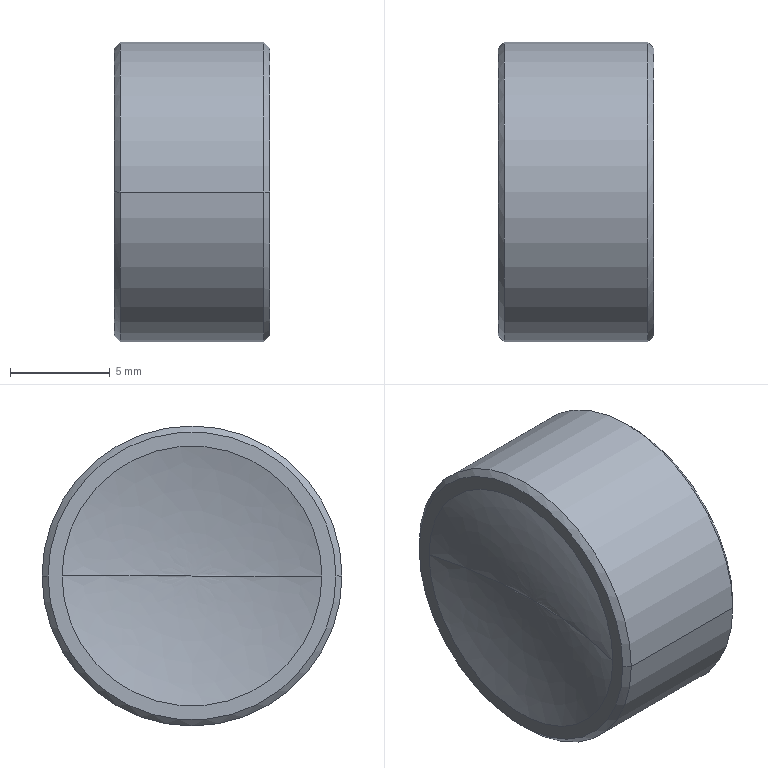Part | STEP file | biconcave lens 4.stp.STEP-235.STEP | 1 solid | 12 faces | box 7.786 x 15 x 15 mm | volume 1252 mm3 | cone 4 | spline 2 | sphere 2 | cylinder 2 | plane 2 | commonest cylinder face diameters 15 x2
STEP:
#1=CARTESIAN_POINT('',(413.933,-0.000000003,0.));
#2=VERTEX_POINT('',#1);
#3=CARTESIAN_POINT('',(413.04,-6.5,0.));
#4=VERTEX_POINT('',#3);
#5=CARTESIAN_POINT('',(413.933,-0.000000003,0.));
#6=CARTESIAN_POINT('',(413.933,-2.201,0.));
#7=CARTESIAN_POINT('',(413.633,-4.381,0.));
#8=CARTESIAN_POINT('',(413.04,-6.5,0.));
#9=(BOUNDED_CURVE()B_SPLINE_CURVE(3,(#5,#6,#7,#8),.UNSPECIFIED.,.F.,.T.)B_SPLINE_CURVE_WITH_KNOTS((4,4),(0.,6.283),.UNSPECIFIED.)CURVE()GEOMETRIC_REPRESENTATION_ITEM()RATIONAL_B_SPLINE_CURVE((1.,0.9938,0.9938,1.))REPRESENTATION_ITEM(''));
#10=EDGE_CURVE('',#2,#4,#9,.T.);
#11=ORIENTED_EDGE('',*,*,#10,.F.);
#12=CARTESIAN_POINT('',(413.04,6.5,0.));
#13=VERTEX_POINT('',#12);
#14=CARTESIAN_POINT('',(413.933,-0.000000003,0.));
#15=CARTESIAN_POINT('',(413.933,2.201,0.));
#16=CARTESIAN_POINT('',(413.633,4.381,0.));
#17=CARTESIAN_POINT('',(413.04,6.5,0.));
#18=(BOUNDED_CURVE()B_SPLINE_CURVE(3,(#14,#15,#16,#17),.UNSPECIFIED.,.F.,.F.)B_SPLINE_CURVE_WITH_KNOTS((4,4),(0.,6.283),.UNSPECIFIED.)CURVE()GEOMETRIC_REPRESENTATION_ITEM()RATIONAL_B_SPLINE_CURVE((1.,0.9938,0.9938,1.))REPRESENTATION_ITEM(''));
#19=EDGE_CURVE('',#2,#13,#18,.T.);
#20=ORIENTED_EDGE('',*,*,#19,.T.);
#21=CARTESIAN_POINT('',(413.04,0.,0.));
#22=DIRECTION('',(1.,0.,0.));
#23=DIRECTION('',(0.,-1.,0.));
#24=AXIS2_PLACEMENT_3D('',#21,#22,#23);
#25=CIRCLE('',#24,6.5);
#26=EDGE_CURVE('',#4,#13,#25,.T.);
#27=ORIENTED_EDGE('',*,*,#26,.F.);
#28=EDGE_LOOP('',(#11,#20,#27));
#29=FACE_OUTER_BOUND('',#28,.T.);
#30=CARTESIAN_POINT('',(413.933,0.,0.));
#31=CARTESIAN_POINT('',(413.933,0.,0.));
#32=CARTESIAN_POINT('',(413.933,0.,0.));
#33=CARTESIAN_POINT('',(413.933,0.,0.));
#34=CARTESIAN_POINT('',(413.933,-2.201,0.));
#35=CARTESIAN_POINT('',(413.933,-2.201,-4.401));
#36=CARTESIAN_POINT('',(413.933,2.201,-4.401));
#37=CARTESIAN_POINT('',(413.933,2.201,0.));
#38=CARTESIAN_POINT('',(413.633,-4.381,0.));
#39=CARTESIAN_POINT('',(413.633,-4.381,-8.762));
#40=CARTESIAN_POINT('',(413.633,4.381,-8.762));
#41=CARTESIAN_POINT('',(413.633,4.381,0.));
#42=CARTESIAN_POINT('',(413.04,-6.5,0.));
#43=CARTESIAN_POINT('',(413.04,-6.5,-13.));
#44=CARTESIAN_POINT('',(413.04,6.5,-13.));
#45=CARTESIAN_POINT('',(413.04,6.5,0.));
#46=(BOUNDED_SURFACE()B_SPLINE_SURFACE(3,3,((#30,#31,#32,#33),(#34,#35,#36,#37),(#38,#39,#40,#41),(#42,#43,#44,#45)),.UNSPECIFIED.,.F.,.F.,.T.)B_SPLINE_SURFACE_WITH_KNOTS((4,4),(4,4),(0.,6.283),(1.298,1.434),.UNSPECIFIED.)GEOMETRIC_REPRESENTATION_ITEM()RATIONAL_B_SPLINE_SURFACE(((1.,0.3333,0.3333,1.),(0.9938,0.3313,0.3313,0.9938),(0.9938,0.3313,0.3313,0.9938),(1.,0.3333,0.3333,1.)))REPRESENTATION_ITEM('')SURFACE());
#47=ADVANCED_FACE('',(#29),#46,.F.);
#48=CARTESIAN_POINT('',(420.826,6.5,0.));
#49=VERTEX_POINT('',#48);
#50=CARTESIAN_POINT('',(420.826,-6.5,0.));
#51=VERTEX_POINT('',#50);
#52=CARTESIAN_POINT('',(444.032,0.,0.));
#53=DIRECTION('',(0.,0.,1.));
#54=DIRECTION('',(0.,-1.,0.));
#55=AXIS2_PLACEMENT_3D('',#52,#53,#54);
#56=CIRCLE('',#55,24.099);
#57=EDGE_CURVE('',#49,#51,#56,.T.);
#58=ORIENTED_EDGE('',*,*,#57,.F.);
#59=CARTESIAN_POINT('',(420.826,0.,0.));
#60=DIRECTION('',(1.,0.,0.));
#61=DIRECTION('',(0.,-1.,0.));
#62=AXIS2_PLACEMENT_3D('',#59,#60,#61);
#63=CIRCLE('',#62,6.5);
#64=EDGE_CURVE('',#49,#51,#63,.T.);
#65=ORIENTED_EDGE('',*,*,#64,.T.);
#66=EDGE_LOOP('',(#58,#65));
#67=FACE_OUTER_BOUND('',#66,.T.);
#68=CARTESIAN_POINT('',(444.032,0.,0.));
#69=DIRECTION('',(0.,0.,1.));
#70=DIRECTION('',(0.,-1.,0.));
#71=AXIS2_PLACEMENT_3D('',#68,#69,#70);
#72=SPHERICAL_SURFACE('',#71,24.099);
#73=ADVANCED_FACE('',(#67),#72,.F.);
#74=CARTESIAN_POINT('',(420.826,7.2,0.));
#75=VERTEX_POINT('',#74);
#76=CARTESIAN_POINT('',(420.826,-7.2,0.));
#77=VERTEX_POINT('',#76);
#78=CARTESIAN_POINT('',(420.826,0.,0.));
#79=DIRECTION('',(1.,0.,0.));
#80=DIRECTION('',(0.,1.,0.));
#81=AXIS2_PLACEMENT_3D('',#78,#79,#80);
#82=CIRCLE('',#81,7.2);
#83=EDGE_CURVE('',#75,#77,#82,.T.);
#84=ORIENTED_EDGE('',*,*,#83,.F.);
#85=CARTESIAN_POINT('',(420.526,7.5,0.));
#86=VERTEX_POINT('',#85);
#87=CARTESIAN_POINT('',(420.826,7.2,0.));
#88=DIRECTION('',(-0.7071,0.7071,0.));
#89=VECTOR('',#88,1000.);
#90=LINE('',#87,#89);
#91=EDGE_CURVE('',#75,#86,#90,.T.);
#92=ORIENTED_EDGE('',*,*,#91,.T.);
#93=CARTESIAN_POINT('',(420.526,-7.5,0.));
#94=VERTEX_POINT('',#93);
#95=CARTESIAN_POINT('',(420.526,0.,0.));
#96=DIRECTION('',(-1.,0.,0.));
#97=DIRECTION('',(0.,1.,0.));
#98=AXIS2_PLACEMENT_3D('',#95,#96,#97);
#99=CIRCLE('',#98,7.5);
#100=EDGE_CURVE('',#94,#86,#99,.T.);
#101=ORIENTED_EDGE('',*,*,#100,.F.);
#102=CARTESIAN_POINT('',(420.826,-7.2,0.));
#103=DIRECTION('',(-0.7071,-0.7071,0.));
#104=VECTOR('',#103,1000.);
#105=LINE('',#102,#104);
#106=EDGE_CURVE('',#77,#94,#105,.T.);
#107=ORIENTED_EDGE('',*,*,#106,.F.);
#108=EDGE_LOOP('',(#84,#92,#101,#107));
#109=FACE_OUTER_BOUND('',#108,.T.);
#110=CARTESIAN_POINT('',(420.826,0.,0.));
#111=DIRECTION('',(-1.,0.,0.));
#112=DIRECTION('',(0.,-1.,0.));
#113=AXIS2_PLACEMENT_3D('',#110,#111,#112);
#114=CONICAL_SURFACE('',#113,7.2,0.7854);
#115=ADVANCED_FACE('',(#109),#114,.T.);
#116=CARTESIAN_POINT('',(413.04,-7.2,0.));
#117=VERTEX_POINT('',#116);
#118=CARTESIAN_POINT('',(413.04,7.2,0.));
#119=VERTEX_POINT('',#118);
#120=CARTESIAN_POINT('',(413.04,0.,0.));
#121=DIRECTION('',(-1.,0.,0.));
#122=DIRECTION('',(0.,-1.,0.));
#123=AXIS2_PLACEMENT_3D('',#120,#121,#122);
#124=CIRCLE('',#123,7.2);
#125=EDGE_CURVE('',#117,#119,#124,.T.);
#126=ORIENTED_EDGE('',*,*,#125,.F.);
#127=CARTESIAN_POINT('',(413.34,-7.5,0.));
#128=VERTEX_POINT('',#127);
#129=CARTESIAN_POINT('',(413.34,-7.5,0.));
#130=DIRECTION('',(0.7071,-0.7071,0.));
#131=VECTOR('',#130,1000.);
#132=LINE('',#129,#131);
#133=EDGE_CURVE('',#117,#128,#132,.T.);
#134=ORIENTED_EDGE('',*,*,#133,.T.);
#135=CARTESIAN_POINT('',(413.34,7.5,0.));
#136=VERTEX_POINT('',#135);
#137=CARTESIAN_POINT('',(413.34,0.,0.));
#138=DIRECTION('',(1.,0.,0.));
#139=DIRECTION('',(0.,-1.,0.));
#140=AXIS2_PLACEMENT_3D('',#137,#138,#139);
#141=CIRCLE('',#140,7.5);
#142=EDGE_CURVE('',#136,#128,#141,.T.);
#143=ORIENTED_EDGE('',*,*,#142,.F.);
#144=CARTESIAN_POINT('',(413.34,7.5,0.));
#145=DIRECTION('',(0.7071,0.7071,0.));
#146=VECTOR('',#145,1000.);
#147=LINE('',#144,#146);
#148=EDGE_CURVE('',#119,#136,#147,.T.);
#149=ORIENTED_EDGE('',*,*,#148,.F.);
#150=EDGE_LOOP('',(#126,#134,#143,#149));
#151=FACE_OUTER_BOUND('',#150,.T.);
#152=CARTESIAN_POINT('',(413.34,0.,0.));
#153=DIRECTION('',(1.,0.,0.));
#154=DIRECTION('',(0.,1.,0.));
#155=AXIS2_PLACEMENT_3D('',#152,#153,#154);
#156=CONICAL_SURFACE('',#155,7.5,0.7854);
#157=ADVANCED_FACE('',(#151),#156,.T.);
#158=CARTESIAN_POINT('',(413.34,0.,0.));
#159=DIRECTION('',(1.,0.,0.));
#160=DIRECTION('',(0.,-1.,0.));
#161=AXIS2_PLACEMENT_3D('',#158,#159,#160);
#162=CIRCLE('',#161,7.5);
#163=EDGE_CURVE('',#128,#136,#162,.T.);
#164=ORIENTED_EDGE('',*,*,#163,.T.);
#165=CARTESIAN_POINT('',(0.,7.5,0.));
#166=DIRECTION('',(1.,0.,0.));
#167=VECTOR('',#166,1000.);
#168=LINE('',#165,#167);
#169=EDGE_CURVE('',#136,#86,#168,.T.);
#170=ORIENTED_EDGE('',*,*,#169,.T.);
#171=CARTESIAN_POINT('',(420.526,0.,0.));
#172=DIRECTION('',(-1.,0.,0.));
#173=DIRECTION('',(0.,1.,0.));
#174=AXIS2_PLACEMENT_3D('',#171,#172,#173);
#175=CIRCLE('',#174,7.5);
#176=EDGE_CURVE('',#86,#94,#175,.T.);
#177=ORIENTED_EDGE('',*,*,#176,.T.);
#178=CARTESIAN_POINT('',(0.,-7.5,0.));
#179=DIRECTION('',(1.,0.,0.));
#180=VECTOR('',#179,1000.);
#181=LINE('',#178,#180);
#182=EDGE_CURVE('',#128,#94,#181,.T.);
#183=ORIENTED_EDGE('',*,*,#182,.F.);
#184=EDGE_LOOP('',(#164,#170,#177,#183));
#185=FACE_OUTER_BOUND('',#184,.T.);
#186=CARTESIAN_POINT('',(0.,0.,0.));
#187=DIRECTION('',(1.,0.,0.));
#188=DIRECTION('',(0.,-1.,0.));
#189=AXIS2_PLACEMENT_3D('',#186,#187,#188);
#190=CYLINDRICAL_SURFACE('',#189,7.5);
#191=ADVANCED_FACE('',(#185),#190,.T.);
#192=ORIENTED_EDGE('',*,*,#26,.T.);
#193=CARTESIAN_POINT('',(413.04,0.,0.));
#194=DIRECTION('',(1.,0.,0.));
#195=DIRECTION('',(0.,-1.,0.));
#196=AXIS2_PLACEMENT_3D('',#193,#194,#195);
#197=CIRCLE('',#196,6.5);
#198=EDGE_CURVE('',#13,#4,#197,.T.);
#199=ORIENTED_EDGE('',*,*,#198,.T.);
#200=EDGE_LOOP('',(#192,#199));
#201=FACE_BOUND('',#200,.T.);
#202=CARTESIAN_POINT('',(413.04,0.,0.));
#203=DIRECTION('',(-1.,0.,0.));
#204=DIRECTION('',(0.,-1.,0.));
#205=AXIS2_PLACEMENT_3D('',#202,#203,#204);
#206=CIRCLE('',#205,7.2);
#207=EDGE_CURVE('',#119,#117,#206,.T.);
#208=ORIENTED_EDGE('',*,*,#207,.T.);
#209=ORIENTED_EDGE('',*,*,#125,.T.);
#210=EDGE_LOOP('',(#208,#209));
#211=FACE_OUTER_BOUND('',#210,.T.);
#212=CARTESIAN_POINT('',(413.04,7.5,0.));
#213=DIRECTION('',(-1.,0.,0.));
#214=DIRECTION('',(0.,1.,0.));
#215=AXIS2_PLACEMENT_3D('',#212,#213,#214);
#216=PLANE('',#215);
#217=ADVANCED_FACE('',(#201,#211),#216,.T.);
#218=ORIENTED_EDGE('',*,*,#169,.F.);
#219=ORIENTED_EDGE('',*,*,#142,.T.);
#220=ORIENTED_EDGE('',*,*,#182,.T.);
#221=ORIENTED_EDGE('',*,*,#100,.T.);
#222=EDGE_LOOP('',(#218,#219,#220,#221));
#223=FACE_OUTER_BOUND('',#222,.T.);
#224=CARTESIAN_POINT('',(0.,0.,0.));
#225=DIRECTION('',(1.,0.,0.));
#226=DIRECTION('',(0.,-1.,0.));
#227=AXIS2_PLACEMENT_3D('',#224,#225,#226);
#228=CYLINDRICAL_SURFACE('',#227,7.5);
#229=ADVANCED_FACE('',(#223),#228,.T.);
#230=ORIENTED_EDGE('',*,*,#19,.F.);
#231=ORIENTED_EDGE('',*,*,#10,.T.);
#232=ORIENTED_EDGE('',*,*,#198,.F.);
#233=EDGE_LOOP('',(#230,#231,#232));
#234=FACE_OUTER_BOUND('',#233,.T.);
#235=CARTESIAN_POINT('',(413.933,0.,0.));
#236=CARTESIAN_POINT('',(413.933,0.,0.));
#237=CARTESIAN_POINT('',(413.933,0.,0.));
#238=CARTESIAN_POINT('',(413.933,0.,0.));
#239=CARTESIAN_POINT('',(413.933,2.201,0.));
#240=CARTESIAN_POINT('',(413.933,2.201,4.401));
#241=CARTESIAN_POINT('',(413.933,-2.201,4.401));
#242=CARTESIAN_POINT('',(413.933,-2.201,0.));
#243=CARTESIAN_POINT('',(413.633,4.381,0.));
#244=CARTESIAN_POINT('',(413.633,4.381,8.762));
#245=CARTESIAN_POINT('',(413.633,-4.381,8.762));
#246=CARTESIAN_POINT('',(413.633,-4.381,0.));
#247=CARTESIAN_POINT('',(413.04,6.5,0.));
#248=CARTESIAN_POINT('',(413.04,6.5,13.));
#249=CARTESIAN_POINT('',(413.04,-6.5,13.));
#250=CARTESIAN_POINT('',(413.04,-6.5,0.));
#251=(BOUNDED_SURFACE()B_SPLINE_SURFACE(3,3,((#235,#236,#237,#238),(#239,#240,#241,#242),(#243,#244,#245,#246),(#247,#248,#249,#250)),.UNSPECIFIED.,.F.,.F.,.T.)B_SPLINE_SURFACE_WITH_KNOTS((4,4),(4,4),(0.,6.283),(1.434,1.571),.UNSPECIFIED.)GEOMETRIC_REPRESENTATION_ITEM()RATIONAL_B_SPLINE_SURFACE(((1.,0.3333,0.3333,1.),(0.9938,0.3313,0.3313,0.9938),(0.9938,0.3313,0.3313,0.9938),(1.,0.3333,0.3333,1.)))REPRESENTATION_ITEM('')SURFACE());
#252=ADVANCED_FACE('',(#234),#251,.F.);
#253=ORIENTED_EDGE('',*,*,#133,.F.);
#254=ORIENTED_EDGE('',*,*,#207,.F.);
#255=ORIENTED_EDGE('',*,*,#148,.T.);
#256=ORIENTED_EDGE('',*,*,#163,.F.);
#257=EDGE_LOOP('',(#253,#254,#255,#256));
#258=FACE_OUTER_BOUND('',#257,.T.);
#259=CARTESIAN_POINT('',(413.34,0.,0.));
#260=DIRECTION('',(1.,0.,0.));
#261=DIRECTION('',(0.,1.,0.));
#262=AXIS2_PLACEMENT_3D('',#259,#260,#261);
#263=CONICAL_SURFACE('',#262,7.5,0.7854);
#264=ADVANCED_FACE('',(#258),#263,.T.);
#265=ORIENTED_EDGE('',*,*,#91,.F.);
#266=CARTESIAN_POINT('',(420.826,0.,0.));
#267=DIRECTION('',(1.,0.,0.));
#268=DIRECTION('',(0.,1.,0.));
#269=AXIS2_PLACEMENT_3D('',#266,#267,#268);
#270=CIRCLE('',#269,7.2);
#271=EDGE_CURVE('',#77,#75,#270,.T.);
#272=ORIENTED_EDGE('',*,*,#271,.F.);
#273=ORIENTED_EDGE('',*,*,#106,.T.);
#274=ORIENTED_EDGE('',*,*,#176,.F.);
#275=EDGE_LOOP('',(#265,#272,#273,#274));
#276=FACE_OUTER_BOUND('',#275,.T.);
#277=CARTESIAN_POINT('',(420.826,0.,0.));
#278=DIRECTION('',(-1.,0.,0.));
#279=DIRECTION('',(0.,-1.,0.));
#280=AXIS2_PLACEMENT_3D('',#277,#278,#279);
#281=CONICAL_SURFACE('',#280,7.2,0.7854);
#282=ADVANCED_FACE('',(#276),#281,.T.);
#283=CARTESIAN_POINT('',(420.826,0.,0.));
#284=DIRECTION('',(1.,0.,0.));
#285=DIRECTION('',(0.,-1.,0.));
#286=AXIS2_PLACEMENT_3D('',#283,#284,#285);
#287=CIRCLE('',#286,6.5);
#288=EDGE_CURVE('',#51,#49,#287,.T.);
#289=ORIENTED_EDGE('',*,*,#288,.F.);
#290=ORIENTED_EDGE('',*,*,#64,.F.);
#291=EDGE_LOOP('',(#289,#290));
#292=FACE_BOUND('',#291,.T.);
#293=ORIENTED_EDGE('',*,*,#271,.T.);
#294=ORIENTED_EDGE('',*,*,#83,.T.);
#295=EDGE_LOOP('',(#293,#294));
#296=FACE_OUTER_BOUND('',#295,.T.);
#297=CARTESIAN_POINT('',(420.826,6.5,0.));
#298=DIRECTION('',(1.,0.,0.));
#299=DIRECTION('',(0.,1.,0.));
#300=AXIS2_PLACEMENT_3D('',#297,#298,#299);
#301=PLANE('',#300);
#302=ADVANCED_FACE('',(#292,#296),#301,.T.);
#303=ORIENTED_EDGE('',*,*,#288,.T.);
#304=ORIENTED_EDGE('',*,*,#57,.T.);
#305=EDGE_LOOP('',(#303,#304));
#306=FACE_OUTER_BOUND('',#305,.T.);
#307=CARTESIAN_POINT('',(444.032,0.,0.));
#308=DIRECTION('',(0.,0.,1.));
#309=DIRECTION('',(0.,-1.,0.));
#310=AXIS2_PLACEMENT_3D('',#307,#308,#309);
#311=SPHERICAL_SURFACE('',#310,24.099);
#312=ADVANCED_FACE('',(#306),#311,.F.);
#313=CLOSED_SHELL('',(#47,#73,#115,#157,#191,#217,#229,#252,#264,#282,#302,#312));
#314=MANIFOLD_SOLID_BREP('',#313);
#315=CARTESIAN_POINT('',(0.,0.,0.));
#316=DIRECTION('',(0.,0.,1.));
#317=DIRECTION('',(1.,0.,0.));
#318=AXIS2_PLACEMENT_3D('',#315,#316,#317);
#319=(LENGTH_UNIT()NAMED_UNIT(*)SI_UNIT(.MILLI.,.METRE.));
#320=UNCERTAINTY_MEASURE_WITH_UNIT(LENGTH_MEASURE(0.00001),#319,'','');
#321=(NAMED_UNIT(*)PLANE_ANGLE_UNIT()SI_UNIT($,.RADIAN.));
#322=(NAMED_UNIT(*)SI_UNIT($,.STERADIAN.)SOLID_ANGLE_UNIT());
#323=(GEOMETRIC_REPRESENTATION_CONTEXT(3)GLOBAL_UNCERTAINTY_ASSIGNED_CONTEXT((#320))GLOBAL_UNIT_ASSIGNED_CONTEXT((#319,#321,#322))REPRESENTATION_CONTEXT('',''));
#324=ADVANCED_BREP_SHAPE_REPRESENTATION('',(#314,#318),#323);